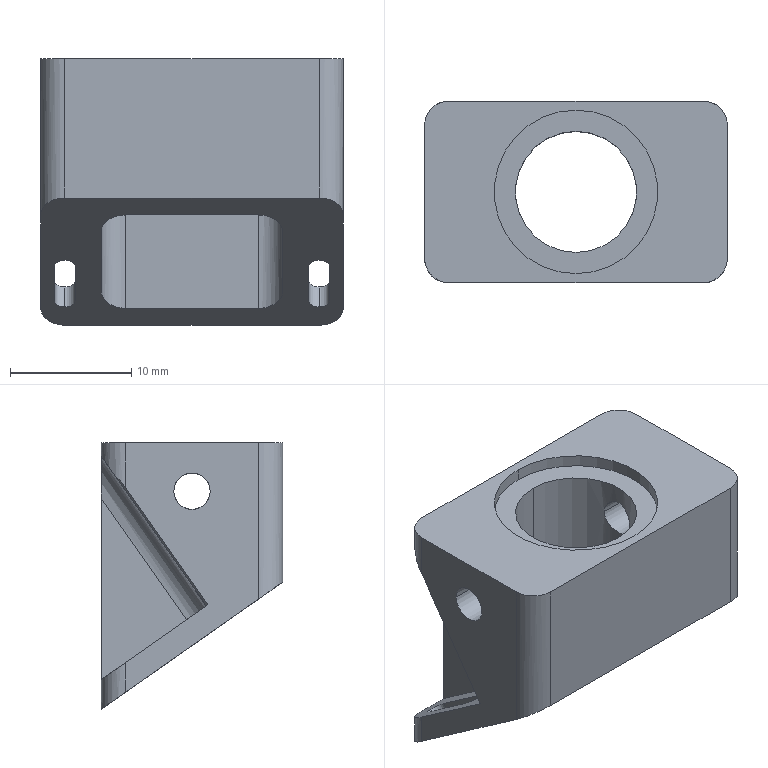NC program | NX | posted with a generic post | part box 25 x 15 x 22 mm
Whole program, first 1577 of 1758 lines:
N10 G17 G21 G94 G90
(FACE_MILLING , TOOL : D40面刀)
N12 T01 M6
N14 G54
N16 G17 G0 G90 X34.5 Y0. S3500 M3
N18 G43 Z20. H1
N20 Z3.
N22 G94 G1 Z0. F480.
N24 X32.5
N26 X-32.5 F800.
N28 X-34.5
N30 Z3.
N32 G0 Z20.
N34 M5
(SPOT_DRILLING , TOOL : D4点钻)
N36 T04 M6
N38 G54
N40 G17 G0 G90 X0. Y0. S2000 M3
N42 G43 Z20. H4
N44 G94 G82 G99 Z-2. F250. P200 R2.
N46 G80
N48 G0 X0. Y0. Z20.
N50 M5
(SPOT_DRILLING_COPY , TOOL : 9.5钻头)
N52 T05 M6
N54 G54
N56 G17 G0 G90 X0. Y0. S1600 M3
N58 G43 Z20. H5
N60 G94 G83 G98 Z-25. F250. Q3. R2.
N62 G80
N64 G0 X0. Y0. Z20.
N66 M5
(PLANAR_MILL , TOOL : D8开粗)
N68 T02 M6
N70 G54
N72 G17 G0 G90 X-21.239 Y-8.5 S4500 M3
N74 G43 Z20. H2
N76 Z-20.3
N78 G94 G1 Z-22.3 F900.
N80 X-20.65
N82 G3 X-17.65 Y-5.5 R3.
N84 G1 Y5.5 F1500.
N86 G2 X-10.5 Y12.65 R7.15
N88 G1 X10.5
N90 G2 X17.65 Y5.5 R7.15
N92 G1 Y-5.5
N94 G2 X10.5 Y-12.65 R7.15
N96 G1 X-10.5
N98 G2 X-17.65 Y-5.5 R7.15
N100 G3 X-20.65 Y-2.5 R3.
N102 G1 X-19.65 Y-8.5
N104 G3 X-16.65 Y-5.5 R3. F900.
N106 G1 Y5.5 F1500.
N108 G2 X-10.5 Y11.65 R6.15
N110 G1 X10.5
N112 G2 X16.65 Y5.5 R6.15
N114 G1 Y-5.5
N116 G2 X10.5 Y-11.65 R6.15
N118 G1 X-10.5
N120 G2 X-16.65 Y-5.5 R6.15
N122 G3 X-19.65 Y-2.5 R3.
N124 G1 X-21.65
N126 Z-20.3
N128 G0 Z20.
(PLANAR_MILL_COPY_2 , TOOL : D8开粗)
N130 X0. Y0.
N132 Z-0.9
N134 G1 X-1.247 Y0.069 F600.
N136 G3 X-2.116 Y-1.511 R1.
N138 X1.511 Y-2.116 R2.6 F1000.
N140 X-2.116 Y-1.511 R-2.6
N142 X-0.34 Y-1.202 R1.
N144 G1 X0. Y0.
N146 G0 Z20.
N148 M5
(PLANAR_MILL_COPY_1 , TOOL : D8精光)
N150 T03 M6
N152 G54
N154 G17 G0 G90 X-20.236 Y-8.465 S4500 M3
N156 G43 Z20. H3
N158 Z-20.3
N160 G94 G1 Z-22.3 F480.
N162 G41 X-20.039 Y-8.5 D3
N164 X-19.5
N166 G3 X-16.5 Y-5.5 R3.
N168 G1 Y5.5 F800.
N170 G2 X-10.5 Y11.5 R6.
N172 G1 X10.5
N174 G2 X16.5 Y5.5 R6.
N176 G1 Y-5.5
N178 G2 X10.5 Y-11.5 R6.
N180 G1 X-10.5
N182 G2 X-16.5 Y-5.5 R6.
N184 G3 X-19.5 Y-2.5 R3.
N186 G1 X-20.5
N188 G40
N190 X-20.697 Y-2.535
N192 Z-20.3
N194 G0 Z20.
(PLANAR_MILL_COPY_1_COPY , TOOL : D8精光)
N196 X-1.569 Y0.065 S3500
N198 Z1.
N200 G1 Z-1. F480.
N202 G41 X-1.75 Y-0.021
N204 X-2.005 Y-0.203
N206 G3 X-2.238 Y-1.598 R1.
N208 X1.598 Y-2.238 R2.75 F800.
N210 X-2.238 Y-1.598 R-2.75
N212 X-0.843 Y-1.831 R1.
N214 G1 X-0.587 Y-1.648
N216 G40
N218 X-0.447 Y-1.506
N220 Z1.
N222 G0 Z20.
N224 M5
(PLANAR_MILL_COPY , TOOL : R1)
N226 T13 M6
N228 G54
N230 G17 G0 G90 X-14.363 Y-6.465 S4500 M3
N232 G43 Z20. H13
N234 Z0.5
N236 G94 G1 Z-0.5 F600.
N238 G41 X-14.166 Y-6.5 D13
N240 G3 X-13.166 Y-5.5 R1.
N242 G1 Y5.5 F1000.
N244 G2 X-10.5 Y8.166 R2.666
N246 G1 X10.5
N248 G2 X13.166 Y5.5 R2.666
N250 G1 Y-5.5
N252 G2 X10.5 Y-8.166 R2.666
N254 G1 X-10.5
N256 G2 X-13.166 Y-5.5 R2.666
N258 G3 X-14.166 Y-4.5 R1.
N260 G40
N262 G1 X-14.363 Y-4.535
N264 Z0.5
N266 G0 Z20.
(PLANAR_MILL_COPY_COPY , TOOL : R1)
N268 X-4.456 Y-1.997
N270 Z0.5
N272 G1 Z-0.5 F600.
N274 G41 X-4.637 Y-2.083
N276 G3 X-4.869 Y-3.478 R1.
N278 X3.478 Y-4.869 R5.984 F1000.
N280 X-4.869 Y-3.478 R-5.984
N282 X-3.474 Y-3.711 R1.
N284 G40
N286 G1 X-3.334 Y-3.568
N288 Z0.5
N290 G0 Z20.
(PLANAR_MILL_COPY_COPY_COPY , TOOL : R1)
N292 X-2.989 Y-0.949
N294 Z-0.5
N296 G1 Z-1.5 F600.
N298 G41 X-3.169 Y-1.035
N300 X-3.294 Y-1.124
N302 G3 X-3.527 Y-2.519 R1.
N304 X2.519 Y-3.527 R4.334 F1000.
N306 X-3.527 Y-2.519 R-4.334
N308 X-2.132 Y-2.752 R1.
N310 G1 X-2.007 Y-2.662
N312 G40
N314 X-1.867 Y-2.52
N316 Z-0.5
N318 G0 Z20.
N320 M5
(ADAPTIVE_MILLING , TOOL : D4开粗)
N322 T08 M6
N324 G54
N326 G17 G0 G90 X-15.582 Y11.515 S5500 M3
N328 G43 Z13.982 H8
N330 Z-12.918
N332 G94 G1 Z-15.918 F1200.
N334 X-15.232 Y11.543 F2000.
N336 X-14.884 Y11.588
N338 G3 X-14.6 Y11.973 R0.405
N340 G2 X-14.386 Y13.882 R6.031
N342 G3 X-14.206 Y17.495 R26.504
N344 G2 X-14.176 Y23.935 R463.382
N346 X-12.751 Y25.861 R2.494
N348 X-9.948 Y26.517 R7.049
N350 G3 X-8.631 Y26.644 R8.532
N352 X-8.035 Y27.2 R0.873
N354 X-8.3 Y27.648 R0.402
N356 G1 X-9.027 Y27.947 Z-15.818
N358 X-9.377 Y28.086
N360 X-9.472 Y28.094
N362 X-9.566 Y28.084
N364 X-12.581 Y27.326
N366 G3 X-13.515 Y26.843 R3.15
N368 X-14.641 Y25.821 R6.151
N370 X-15.3 Y24.545 R4.061
N372 X-15.515 Y23.303 R4.524
N374 G1 X-15.776 Y14.49
N376 X-15.745 Y14.376
N378 X-15.44 Y13.687
N380 X-15.337 Y13.448 Z-15.851
N382 X-15.219 Y13.215 Z-15.884
N384 G3 X-15.006 Y13.067 Z-15.918 R0.413
N386 X-14.528 Y13.299 R0.401
N388 X-13.886 Y16.065 R6.646
N390 X-13.786 Y22.835 R158.507
N392 G2 X-11.974 Y25.361 R3.146
N394 X-9.563 Y26.059 R8.306
N396 G3 X-8.14 Y26.72 R2.469
N398 X-8.021 Y26.99 R0.72
N400 X-8.231 Y27.36 R0.402
N402 X-8.555 Y27.414 Z-15.876 R0.726
N404 G1 X-9.008 Y27.433 Z-15.818
N406 X-9.672 Y27.457
N408 G3 X-11.285 Y27.007 R13.359
N410 G1 X-12.09 Y26.663
N412 X-12.882 Y26.289
N414 G3 X-14.037 Y25.322 R3.789
N416 X-14.633 Y24.272 R3.101
N418 X-14.988 Y22.607 R5.297
N420 G1 X-15.203 Y15.337
N422 X-15.089 Y14.429
N424 X-15.058 Y14.17 Z-15.851
N426 X-15.011 Y13.913 Z-15.884
N428 G3 X-14.849 Y13.711 Z-15.918 R0.413
N430 X-14.319 Y13.806 R0.4
N432 X-13.657 Y15.437 R3.226
N434 X-13.409 Y19.6 R28.394
N436 G2 X-13.352 Y22.236 R29.078
N438 X-11.199 Y24.963 R3.652
N440 X-9.138 Y25.755 R37.205
N442 G3 X-8.062 Y26.523 R2.381
N444 G1 X-8.011 Y26.711
N446 X-8.035 Y27.51
N448 G3 X-8.323 Y27.882 R0.401
N450 X-8.731 Y27.778 Z-15.862 R0.439
N452 G1 X-9.011 Y27.575 Z-15.818
N454 X-9.743 Y27.053
N456 X-11.542 Y26.149
N458 G3 X-12.882 Y25.289 R8.835
N460 X-14.07 Y23.854 R5.135
N462 X-14.46 Y22.55 R3.909
N464 G1 X-14.597 Y21.332
N466 X-14.702 Y20.111
N468 X-15.021 Y15.535
N470 X-14.908 Y14.669
N472 X-14.835 Y14.167 Z-15.882
N474 G3 X-14.668 Y13.95 Z-15.918 R0.421
N476 X-14.136 Y14.044 R0.4
N478 X-13.297 Y15.907 R3.444
N480 X-13.017 Y19.958 R26.017
N482 G2 X-12.835 Y22.037 R7.857
N484 X-10.779 Y24.467 R4.194
N486 G3 X-8.738 Y25.553 R56.293
N488 X-8.016 Y26.28 R1.703
N490 G1 X-8.011 Y26.726
N492 G3 X-8.235 Y27.073 R0.402
N494 X-8.59 Y27.08 Z-15.871 R0.456
N496 G1 X-8.996 Y26.969 Z-15.818
N498 X-9.693 Y26.776
N500 X-9.779 Y26.726
N502 X-12.528 Y24.664
N504 G3 X-13.045 Y24.146 R2.528
N506 G1 X-13.309 Y23.777
N508 X-13.553 Y23.394
N510 G3 X-14.007 Y22.147 R4.286
N512 G1 X-14.119 Y21.57
N514 X-14.203 Y20.989
N516 X-14.8 Y15.787
N518 X-14.664 Y14.962
N520 X-14.573 Y14.461 Z-15.883
N522 G3 X-14.401 Y14.252 Z-15.918 R0.421
N524 X-13.913 Y14.312 R0.401
N526 X-13.062 Y15.769 R2.627
N528 X-12.648 Y19.389 R16.304
N530 G2 X-12.358 Y21.655 R7.242
N532 X-10.332 Y24.068 R4.979
N534 G3 X-9.827 Y24.449 R2.094
N536 G1 X-9.702 Y24.694
N538 X-9.242 Y25.155
N540 G3 X-8.192 Y25.755 R4.982
N542 X-8.002 Y26.419 R0.706
N544 X-8.827 Y26.619 R0.44
N546 G1 X-9.144 Y26.034
N548 G3 X-8.661 Y25.45 R0.44
N550 X-7.998 Y25.905 R0.683
N552 G1 X-7.995 Y26.169
N554 G3 X-8.812 Y26.381 R0.44
N556 G1 X-8.991 Y26.07
N558 G3 X-8.513 Y25.474 R0.44
N560 X-7.989 Y25.983 R0.482
N562 X-8.208 Y26.328 R0.402
N564 G1 X-8.364 Y26.373 Z-15.897
N566 X-8.524 Y26.394 Z-15.877
N568 X-8.981 Y26.458 Z-15.818
N570 X-9.464 Y26.52
N572 G3 X-9.697 Y26.44 R0.421
N574 G1 X-11.459 Y25.112
N576 G3 X-12.701 Y23.628 R5.464
N578 X-13.537 Y21.863 R8.092
N580 X-13.73 Y20.909 R5.162
N582 G1 X-14.214 Y16.147
N584 X-14.336 Y15.254
N586 X-14.374 Y14.996 Z-15.851
N588 X-14.396 Y14.736 Z-15.884
N590 G3 X-14.292 Y14.499 Z-15.918 R0.413
N592 X-13.755 Y14.452 R0.4
N594 X-12.779 Y15.863 R2.479
N596 X-12.305 Y18.84 R12.275
N598 G2 X-11.91 Y21.242 R7.668
N600 X-10.315 Y23.409 R5.937
N602 G3 X-9.998 Y24.113 R0.903
N604 G1 X-9.816 Y24.47
N606 G3 X-10.622 Y24.821 R-0.44
N608 G1 X-10.798 Y24.339
N610 X-11.068 Y23.601 Z-15.818
N612 X-14.044 Y15.477
N614 X-14.12 Y15.277 Z-15.845
N616 X-14.18 Y15.071 Z-15.872
N618 G3 X-14.087 Y14.738 Z-15.918 R0.444
N620 X-13.477 Y14.665 R0.44
N622 X-12.524 Y15.881 R2.225
N624 X-11.983 Y18.413 R9.705
N626 G2 X-11.402 Y21.032 R7.915
N628 X-10.256 Y22.791 R10.278
N630 G3 X-10.1 Y23.471 R0.899
N632 G1 X-10.053 Y23.767
N634 G3 X-10.755 Y24.185 R0.44
N636 X-10.94 Y23.874 Z-15.871 R0.583
N638 G1 X-11.078 Y23.481 Z-15.818
N640 X-13.825 Y15.618
N642 X-13.899 Y15.413 Z-15.846
N644 X-13.958 Y15.203 Z-15.873
N646 G3 X-13.866 Y14.876 Z-15.918 R0.445
N648 X-13.354 Y14.744 R0.441
N650 X-12.319 Y15.792 R1.908
N652 X-11.665 Y18.152 R8.173
N654 G2 X-10.274 Y21.968 R8.667
N656 G3 X-10.1 Y22.369 R1.883
N658 G1 Y23.169
N660 G3 X-10.666 Y23.591 R0.44
N662 X-10.98 Y23.245 Z-15.856 R0.474
N664 G1 X-11.078 Y22.964 Z-15.818
N666 X-13.638 Y15.698
N668 X-13.713 Y15.492 Z-15.846
N670 X-13.773 Y15.281 Z-15.874
N672 G3 X-13.684 Y14.956 Z-15.918 R0.445
N674 X-13.169 Y14.82 R0.441
N676 X-12.022 Y15.894 R2.011
N678 X-11.425 Y17.627 R7.32
N680 G2 X-10.131 Y21.34 R13.088
N682 G3 X-10.1 Y22.37 R4.674
N684 X-10.674 Y22.789 R0.44
N686 X-10.98 Y22.442 Z-15.856 R0.475
N688 G1 X-11.078 Y22.157 Z-15.818
N690 X-13.248 Y15.859
N692 X-13.328 Y15.638 Z-15.848
N694 X-13.388 Y15.411 Z-15.878
N696 G3 X-13.307 Y15.113 Z-15.918 R0.447
N698 X-12.894 Y14.934 R0.442
N700 X-11.949 Y15.626 R1.519
N702 X-11.067 Y17.679 R6.627
N704 G2 X-10.105 Y20.411 R25.158
N706 G1 X-10.1 Y21.496
N708 G3 X-10.638 Y21.925 R0.44
N710 X-10.976 Y21.588 Z-15.854 R0.47
N712 G1 X-11.078 Y21.323 Z-15.818
N714 X-13.178 Y15.882
N716 X-13.267 Y15.662 Z-15.848
N718 X-13.336 Y15.435 Z-15.878
N720 G3 X-13.271 Y15.138 Z-15.918 R0.448
N722 X-12.844 Y14.941 R0.442
N724 X-11.671 Y15.673 R1.616
N726 X-10.738 Y17.593 R7.135
N728 G1 X-10.1 Y19.345
N730 Y20.495
N732 G3 X-10.609 Y20.93 R0.44
N734 X-10.974 Y20.598 Z-15.852 R0.471
N736 G1 X-11.078 Y20.354 Z-15.818
N738 X-12.959 Y15.926
N740 X-13.056 Y15.705 Z-15.848
N742 X-13.135 Y15.478 Z-15.879
N744 G3 X-13.085 Y15.185 Z-15.918 R0.449
N746 X-12.646 Y14.967 R0.441
N748 X-11.405 Y15.688 R1.707
N750 X-10.252 Y17.877 R8.845
N752 G1 X-10.1 Y18.301
N754 Y19.351
N756 G3 X-10.57 Y19.79 R0.44
N758 X-10.967 Y19.479 Z-15.85 R0.467
N760 G1 X-11.078 Y19.252 Z-15.818
N762 X-12.688 Y15.96
N764 X-12.795 Y15.75 Z-15.848
N766 X-12.883 Y15.531 Z-15.878
N768 G3 X-12.843 Y15.228 Z-15.918 R0.448
N770 X-12.398 Y15. R0.441
N772 X-11.204 Y15.615 R1.625
N774 X-10.107 Y17.404 R6.423
N776 G1 X-10.1 Y18.303
N778 G3 X-10.516 Y18.742 R0.44
N780 X-10.957 Y18.463 Z-15.847 R0.469
N782 G1 X-11.076 Y18.265 Z-15.818
N784 X-12.434 Y15.993
N786 X-12.559 Y15.79 Z-15.848
N788 X-12.667 Y15.578 Z-15.879
N790 G3 X-12.655 Y15.276 Z-15.918 R0.448
N792 X-12.249 Y15.006 R0.441
N794 X-10.978 Y15.562 R1.634
N796 X-10.113 Y16.743 R4.303
N798 G1 X-10.1 Y17.463
N800 G3 X-10.475 Y17.899 R0.441
N802 X-10.941 Y17.659 Z-15.847 R0.468
N804 G1 X-11.075 Y17.474 Z-15.818
N806 X-12.143 Y15.998
N808 X-12.392 Y15.644 Z-15.873
N810 G3 X-12.414 Y15.301 Z-15.918 R0.455
N812 X-11.999 Y15.006 R0.441
N814 X-10.681 Y15.561 R1.759
N816 X-10.11 Y16.291 R1.983
N818 G1 X-10.1 Y16.85
N820 G3 X-10.443 Y17.279 R0.441
N822 X-10.924 Y17.078 Z-15.847 R0.469
N824 G1 X-11.075 Y16.902 Z-15.818
N826 X-11.856 Y15.996
N828 X-12.125 Y15.674 Z-15.871
N830 G3 X-12.171 Y15.322 Z-15.918 R0.454
N832 X-11.749 Y15.006 R0.441
N834 X-10.123 Y15.903 R1.813
N836 X-10.1 Y16.358 R3.558
N838 X-10.411 Y16.779 R0.441
N840 X-10.895 Y16.628 Z-15.85 R0.466
N842 G1 X-11.076 Y16.456 Z-15.818
N844 X-11.561 Y15.995
N846 X-11.718 Y15.848 Z-15.845
N848 X-11.864 Y15.69 Z-15.873
N850 G3 X-11.929 Y15.351 Z-15.918 R0.444
N852 X-11.499 Y15.006 R0.441
N854 X-10.127 Y15.64 R1.381
N856 X-10.1 Y16.056 R2.236
N858 X-10.407 Y16.476 R0.441
N860 X-10.892 Y16.33 Z-15.85 R0.467
N862 G1 X-11.076 Y16.16 Z-15.818
N864 X-11.254 Y15.994
N866 X-11.413 Y15.85 Z-15.845
N868 X-11.56 Y15.695 Z-15.872
N870 G3 X-11.63 Y15.355 Z-15.918 R0.444
N872 X-11.199 Y15.006 R0.441
N874 X-10.149 Y15.411 R1.112
N876 X-10.1 Y15.778 R0.942
N878 X-10.839 Y16.101 R0.44
N880 G1 X-11.245 Y15.717
N882 G3 X-10.899 Y15.006 R0.44
N884 X-10.173 Y15.249 R0.793
N886 X-10.1 Y15.607 R0.686
N888 X-10.904 Y15.854 R0.44
N890 G1 X-10.998 Y15.718
N892 X-11.071 Y15.57
N894 G3 X-10.649 Y15.006 R0.44
N896 X-10.1 Y15.481 R0.455
N898 X-10.384 Y15.867 R0.405
N900 G1 X-11.082 Y16.084
N902 Z-12.918
N904 G0 Z13.982
N906 X7.338 Y28.069
N908 Z-12.918
N910 G1 Z-15.918 F1200.
N912 X6.703 Y27.909 F2000.
N914 G3 X6.399 Y27.485 R0.405
N916 X6.856 Y26.906 R0.533
N918 X9.472 Y26.634 R10.905
N920 G2 X11.69 Y26.569 R27.629
N922 X13.507 Y25.066 R2.578
N924 X14.119 Y22.199 R7.582
N926 X14.205 Y14.761 R179.701
N928 G1 X14.301 Y13.849
N930 G2 X14.6 Y12.755 R2.563
N932 G1 Y11.955
N934 G3 X15.274 Y11.664 R0.4
N936 X15.427 Y11.96 Z-15.875 R0.704
N938 G1 X15.579 Y12.382 Z-15.818
N940 X15.717 Y12.757
N942 X15.844 Y13.136
N944 X15.85 Y13.205
N946 X15.853 Y15.046
N948 X15.831 Y16.887
N950 G3 X15.546 Y20.554 R39.884
N952 G1 X15.114 Y23.963
N954 G3 X13.707 Y26.848 R5.665
N956 X12.675 Y27.51 R3.134
N958 X11.352 Y27.85 R5.189
N960 G1 X7.939 Y28.269
N962 X7.836 Y28.266
N964 X7.735 Y28.241
N966 X7.354 Y28.081
N968 X6.629 Y27.776 Z-15.918
N970 G3 X6.408 Y27.385 R0.401
N972 X6.807 Y26.807 R0.604
N974 X8.97 Y26.319 R5.727
N976 G2 X10.79 Y26.182 R20.503
N978 X13.072 Y24.165 R3.335
N980 X13.708 Y21.046 R9.166
N982 X13.812 Y15.325 R146.03
N984 G3 X13.932 Y14.314 R3.116
N986 G1 X14.338 Y13.76
N988 G3 X14.944 Y13.591 R0.4
N990 X15.112 Y13.953 Z-15.865 R0.442
N992 G1 X15.143 Y14.323 Z-15.818
N994 X15.222 Y15.291
N996 X15.202 Y16.722
N998 X15.162 Y18.153
N1000 X15.092 Y19.295
N1002 X14.99 Y20.435
N1004 X14.733 Y22.833
N1006 G3 X13.939 Y25.217 R7.439
N1008 X12.76 Y26.523 R4.348
N1010 X11.491 Y27.244 R5.443
N1012 X10.701 Y27.42 R4.004
N1014 G1 X10.053 Y27.501
N1016 X8.079 Y27.695
N1018 X7.386 Y27.68
N1020 X6.741 Y27.66 Z-15.9
N1022 X6.611 Y27.61 Z-15.918
N1024 G3 X6.42 Y27.235 R0.402
N1026 X6.908 Y26.601 R0.867
N1028 X9.124 Y25.98 R5.46
N1030 G2 X12.668 Y23.407 R3.907
N1032 X13.312 Y19.983 R10.693
N1034 X13.435 Y15.362 R599.298
N1036 G3 X13.629 Y14.558 R1.508
N1038 G1 X13.977 Y14.249
N1040 G3 X14.445 Y14.176 R0.401
N1042 X14.667 Y14.542 Z-15.861 R0.437
N1044 G1 X14.721 Y14.876 Z-15.818
N1046 X14.861 Y15.78
N1048 X14.862 Y16.802
N1050 X14.84 Y17.825
N1052 G3 X14.674 Y19.449 R16.845
N1054 G1 X14.24 Y22.236
N1056 G3 X13.649 Y24.203 R9.935
N1058 G1 X13.306 Y25.009
N1060 G3 X12.39 Y26.04 R2.832
N1062 X10.131 Y27.084 R8.287
N1064 G1 X8.072 Y27.655
N1066 X7.389 Y27.637
N1068 X6.741 Y27.61 Z-15.9
N1070 X6.614 Y27.559 Z-15.918
N1072 G3 X6.424 Y27.186 R0.402
N1074 X6.958 Y26.39 R1.047
N1076 X8.898 Y25.686 R5.264
N1078 G2 X12.312 Y22.635 R4.511
N1080 X12.924 Y18.898 R12.878
N1082 G3 X13.064 Y15.537 R68.24
N1084 X13.289 Y14.809 R1.429
N1086 G1 X13.365 Y14.744
N1088 G3 X13.766 Y14.745 R0.402
N1090 X13.971 Y15.072 Z-15.867 R0.449
N1092 G1 X14.061 Y15.448 Z-15.818
N1094 X14.246 Y16.228
N1096 G3 X14.208 Y18.728 R34.896
N1098 G1 X14.153 Y19.338
N1100 X14.084 Y19.947
N1102 X13.876 Y21.44
N1104 G3 X13.035 Y23.947 R8.586
N1106 X11.818 Y25.582 R7.801
N1108 X10.822 Y26.28 R3.806
N1110 X9.456 Y26.796 R5.492
N1112 G1 X8.164 Y27.096
N1114 X7.407 Y27.348
N1116 X6.896 Y27.513 Z-15.886
N1118 G3 X6.654 Y27.477 Z-15.918 R0.428
N1120 X6.432 Y27.086 R0.401
N1122 X7.037 Y26.131 R1.253
N1124 X8.709 Y25.436 R4.217
N1126 G2 X12.033 Y21.678 R5.414
N1128 X12.541 Y17.82 R16.66
N1130 G3 X12.744 Y15.485 R13.773
N1132 X13.108 Y14.846 R0.936
N1134 G2 X13.678 Y14.511 R1.44
N1136 G3 X14.202 Y14.544 R0.401
N1138 X14.307 Y14.958 Z-15.861 R0.437
N1140 G1 X14.261 Y15.294 Z-15.818
N1142 X13.992 Y17.34
N1144 X13.739 Y19.387
N1146 G3 X13.036 Y22.561 R16.894
N1148 X11.903 Y24.627 R6.798
N1150 X9.573 Y26.347 R6.279
N1152 G1 X8.179 Y26.949
N1154 X7.419 Y27.2
N1156 X6.908 Y27.363 Z-15.886
N1158 X6.784 Z-15.902
N1160 X6.666 Y27.327 Z-15.918
N1162 G3 X6.444 Y26.936 R0.401
N1164 X7.081 Y25.875 R1.383
N1166 X8.019 Y25.552 R1.122
N1168 G1 X8.414 Y25.49
N1170 G3 X8.918 Y25.987 R0.44
N1172 X8.624 Y26.347 Z-15.856 R0.475
N1174 G1 X8.36 Y26.489 Z-15.818
N1176 X7.435 Y26.985
N1178 X7.227 Y27.1 Z-15.848
N1180 X7.01 Y27.197 Z-15.878
N1182 G3 X6.709 Y27.169 Z-15.918 R0.448
N1184 X6.46 Y26.737 R0.441
N1186 X7.257 Y25.563 R1.357
N1188 G1 X7.668 Y25.552
N1190 G3 X8.102 Y25.915 R0.441
N1192 X7.876 Y26.387 Z-15.847 R0.468
N1194 G1 X7.695 Y26.528 Z-15.818
N1196 X7.456 Y26.712
N1198 X7.284 Y26.847 Z-15.846
N1200 X7.103 Y26.97 Z-15.874
N1202 G3 X6.765 Y26.987 Z-15.918 R0.445
N1204 X6.476 Y26.538 R0.441
N1206 X6.972 Y25.586 R1.069
N1208 X7.359 Y25.552 R1.533
N1210 X7.652 Y26.32 R0.44
N1212 G1 X7.168 Y26.744
N1214 G3 X6.492 Y26.338 R0.44
N1216 X6.775 Y25.619 R0.833
N1218 X7.124 Y25.552 R0.719
N1220 X7.392 Y26.341 R0.44
N1222 G1 X7.25 Y26.453
N1224 X7.092 Y26.542
N1226 G3 X6.513 Y26.089 R0.44
N1228 X6.998 Y25.552 R0.469
N1230 G2 X8.661 Y25.45 R6.715
N1232 G1 X9.242 Y25.155
N1234 G2 X11.918 Y19.814 R8.603
N1236 X12.237 Y16.398 R108.189
N1238 G3 X12.649 Y15.075 R3.
N1240 G1 X12.857 Y14.941
N1242 G3 X13.29 Y15.086 R0.442
N1244 X13.353 Y15.571 Z-15.852 R0.474
N1246 G1 X13.275 Y15.831 Z-15.818
N1248 X11.085 Y23.124
N1250 X10.859 Y23.876 Z-15.918
N1252 X10.68 Y24.484
N1254 X10.489 Y25.088
N1256 G3 X9.702 Y24.694 R-0.44
N1258 G2 X11.16 Y21.175 R19.871
N1260 X11.753 Y17.226 R23.84
N1262 G3 X12.19 Y15.386 R5.509
N1264 X12.894 Y14.934 R0.707
N1266 G1 X13.124 Y14.839
N1268 G3 X13.621 Y14.953 R0.441
N1270 X13.69 Y15.449 Z-15.85 R0.468
N1272 G1 X13.612 Y15.693 Z-15.818
N1274 X11.069 Y23.636
N1276 X10.824 Y24.383 Z-15.918
N1278 G3 X9.998 Y24.113 R0.44
N1280 X10.593 Y21.679 R16.069
N1282 G2 X11.345 Y17.319 R29.758
N1284 G3 X11.889 Y15.408 R5.352
N1286 X12.648 Y14.967 R0.793
N1288 X13.063 Y15.145 R0.442
N1290 X13.112 Y15.586 Z-15.859 R0.475
N1292 G1 X13.029 Y15.899 Z-15.818
N1294 X11.085 Y23.203
N1296 X10.929 Y23.766 Z-15.892
N1298 X10.877 Y23.852 Z-15.905
N1300 X10.81 Y23.926 Z-15.918
N1302 G3 X10.092 Y23.521 R0.44
N1304 X10.341 Y21.222 R9.938
N1306 G2 X11.001 Y17.084 R229.932
N1308 G3 X11.702 Y15.259 R4.203
N1310 X12.351 Y15.006 R0.637
N1312 X12.709 Y15.191 R0.443
N1314 X12.761 Y15.622 Z-15.86 R0.479
N1316 G1 X12.682 Y15.947 Z-15.818
N1318 X11.084 Y22.496
N1320 X11.018 Y22.778 Z-15.855
N1322 X10.937 Y23.056 Z-15.892
N1324 X10.882 Y23.142 Z-15.905
N1326 X10.811 Y23.216 Z-15.918
N1328 G3 X10.1 Y22.869 R0.44
N1330 X10.756 Y16.591 R24.263
N1332 X11.576 Y15.096 R2.956
N1334 X12.109 Y15.006 R0.769
N1336 X12.486 Y15.219 R0.442
N1338 X12.513 Y15.637 Z-15.863 R0.488
N1340 G1 X12.421 Y15.977 Z-15.818
N1342 X11.084 Y20.894
N1344 X10.943 Y21.396 Z-15.884
N1346 G3 X10.772 Y21.593 Z-15.918 R0.47
N1348 X10.1 Y21.219 R0.44
N1350 X10.14 Y18.057 R41.425
N1352 X10.925 Y15.477 R5.782
N1354 X11.506 Y15.006 R0.933
N1356 G1 X11.856
N1358 G3 X12.243 Y15.237 R0.442
N1360 X12.236 Y15.679 Z-15.859 R0.476
N1362 G1 X12.113 Y15.98 Z-15.818
N1364 X11.086 Y18.497
N1366 X11. Y18.715 Z-15.848
N1368 X10.895 Y18.926 Z-15.878
N1370 G3 X10.639 Y19.097 Z-15.918 R0.447
N1372 X10.1 Y18.669 R0.44
N1374 X10.148 Y16.743 R13.81
N1376 X10.981 Y15.091 R2.753
N1378 X11.513 Y15.006 R0.8
N1380 X11.91 Y15.257 R0.442
N1382 X11.86 Y15.726 Z-15.855 R0.472
N1384 G1 X11.717 Y15.979 Z-15.818
N1386 X11.087 Y17.094
N1388 X10.983 Y17.282 Z-15.845
N1390 X10.866 Y17.463 Z-15.873
N1392 G3 X10.553 Y17.609 Z-15.918 R0.444
N1394 X10.1 Y17.169 R0.44
N1396 X10.223 Y15.841 R3.676
N1398 X10.798 Y15.045 R1.501
N1400 X11.244 Y15.006 R1.288
N1402 X11.653 Y15.283 R0.441
N1404 X11.556 Y15.766 Z-15.852 R0.471
N1406 G1 X11.4 Y15.982 Z-15.818
N1408 X11.087 Y16.414
N1410 X10.964 Y16.586 Z-15.845
N1412 X10.829 Y16.749 Z-15.872
N1414 G3 X10.494 Y16.856 Z-15.918 R0.444
N1416 X10.1 Y16.419 R0.44
N1418 X10.398 Y15.205 R1.738
N1420 X10.99 Y15.006 R0.63
N1422 X11.406 Y15.303 R0.441
N1424 X11.276 Y15.788 Z-15.85 R0.468
N1426 G1 X11.109 Y15.982 Z-15.818
N1428 X11.088 Y16.007
N1430 X10.95 Y16.169 Z-15.845
N1432 X10.801 Y16.321 Z-15.872
N1434 G3 X10.462 Y16.402 Z-15.918 R0.444
N1436 X10.1 Y15.969 R0.441
N1438 X10.379 Y15.086 R1.022
N1440 X10.75 Y15.006 R0.656
N1442 X11.07 Y15.748 R0.44
N1444 G1 X10.808 Y16.017
N1446 G3 X10.1 Y15.669 R0.44
N1448 X10.39 Y15.037 R0.57
N1450 G1 X10.625 Y15.006
N1452 G3 X10.587 Y15.976 R-0.486
N1454 X10.1 Y15.469 R0.508
N1456 X10.492 Y15.011 R0.426
N1458 X10.942 Y15.291 R0.405
N1460 G1 X11.156 Y15.988
N1462 Z-12.918
N1464 G0 Z13.982
N1466 M5
(PLANAR_MILL_1_COPY , TOOL : D4精刀)
N1468 T06 M6
N1470 G54
N1472 G17 G0 G90 X-16.206 Y11.941 S4500 M3
N1474 G43 Z13.982 H6
N1476 Z-9.018
N1478 G94 G1 Z-10.018 F360.
N1480 G41 X-16.043 Y12.056 D6
N1482 X-13.921 Y14.177
N1484 X-13.771 Y14.327 F600.
N1486 G2 X-12.35 Y14.916 R2.01
N1488 G1 X-10.01
N1490 Y23.506
N1492 Y26.506
N1494 G40
N1496 X-10.045 Y26.703
N1498 Z-9.018
N1500 G0 Z13.982
N1502 X-16.199 Y11.934
N1504 Z-9.018
N1506 G1 Z-10.018 F360.
N1508 G41 X-16.036 Y12.049
N1510 X-13.914 Y14.17
N1512 X-13.764 Y14.32 F600.
N1514 G2 X-12.35 Y14.906 R2.
N1516 G1 X-10.
N1518 Y23.506
N1520 Y26.506
N1522 G40
N1524 X-10.035 Y26.703
N1526 Z-9.018
N1528 G0 Z13.982
N1530 X10.045
N1532 Z-9.018
N1534 G1 Z-10.018 F360.
N1536 G41 X10.01 Y26.506
N1538 Y23.506
N1540 Y14.916 F600.
N1542 X12.35
N1544 G2 X13.771 Y14.327 R2.01
N1546 G1 X13.921 Y14.177
N1548 X16.043 Y12.056
N1550 G40
N1552 X16.206 Y11.941
N1554 Z-9.018
N1556 G0 Z13.982
N1558 X10.035 Y26.703
N1560 Z-9.018
N1562 G1 Z-10.018 F360.
N1564 G41 X10. Y26.506
N1566 Y23.506
N1568 Y14.906 F600.
N1570 X12.35
N1572 G2 X13.764 Y14.32 R2.
N1574 G1 X13.914 Y14.17
N1576 X16.036 Y12.049
N1578 G40
N1580 X16.199 Y11.934
N1582 Z-9.018
N1584 G0 Z13.982
(PLANAR_MILL_1_COPY_COPY , TOOL : D4精刀)
N1586 X-17.614 Y13.348
N1588 Z-15.018
N1590 G1 Z-16.018 F360.
N1592 G41 X-17.45 Y13.463
N1594 X-15.328 Y15.584
N1596 X-15.178 Y15.734 F600.
N1598 G2 X-12.35 Y16.906 R4.
N1600 G1 X-12.
N1602 Y23.506
N1604 Y26.506
N1606 G40
N1608 X-12.035 Y26.703
N1610 Z-15.018
N1612 G0 Z13.982
N1614 X-16.199 Y11.934
N1616 Z-15.018
N1618 G1 Z-16.018 F360.
N1620 G41 X-16.036 Y12.049
N1622 X-13.914 Y14.17
N1624 X-13.764 Y14.32 F600.
N1626 G2 X-12.35 Y14.906 R2.
N1628 G1 X-10.
N1630 Y23.506
N1632 Y26.506
N1634 G40
N1636 X-10.035 Y26.703
N1638 Z-15.018
N1640 G0 Z13.982
N1642 X12.035
N1644 Z-15.018
N1646 G1 Z-16.018 F360.
N1648 G41 X12. Y26.506
N1650 Y23.506
N1652 Y16.906 F600.
N1654 X12.35
N1656 G2 X15.178 Y15.734 R4.
N1658 G1 X15.328 Y15.584
N1660 X17.45 Y13.463
N1662 G40
N1664 X17.614 Y13.348
N1666 Z-15.018
N1668 G0 Z13.982
N1670 X10.035 Y26.703
N1672 Z-15.018
N1674 G1 Z-16.018 F360.
N1676 G41 X10. Y26.506
N1678 Y23.506
N1680 Y14.906 F600.
N1682 X12.35
N1684 G2 X13.764 Y14.32 R2.
N1686 G1 X13.914 Y14.17
N1688 X16.036 Y12.049
N1690 G40
N1692 X16.199 Y11.934
N1694 Z-15.018
N1696 G0 Z13.982
(PLANAR_MILL_1_COPY_COPY_COPY , TOOL : D4精刀)
N1698 X-17.614 Y13.348
N1700 Z-15.018
N1702 G1 Z-16.018 F360.
N1704 G41 X-17.45 Y13.463
N1706 X-15.328 Y15.584
N1708 X-15.178 Y15.734 F600.
N1710 G2 X-12.35 Y16.906 R4.
N1712 G1 X-12.
N1714 Y23.506
N1716 Y26.506
N1718 G40
N1720 X-12.035 Y26.703
N1722 Z-15.018
N1724 G0 Z13.982
N1726 X-16.199 Y11.934
N1728 Z-15.018
N1730 G1 Z-16.018 F360.
N1732 G41 X-16.036 Y12.049
N1734 X-13.914 Y14.17
N1736 X-13.764 Y14.32 F600.
N1738 G2 X-12.35 Y14.906 R2.
N1740 G1 X-10.
N1742 Y23.506
N1744 Y26.506
N1746 G40
N1748 X-10.035 Y26.703
N1750 Z-15.018
N1752 G0 Z13.982
N1754 X12.035
N1756 Z-15.018
N1758 G1 Z-16.018 F360.
N1760 G41 X12. Y26.506
N1762 Y23.506
N1764 Y16.906 F600.
N1766 X12.35
N1768 G2 X15.178 Y15.734 R4.
N1770 G1 X15.328 Y15.584
N1772 X17.45 Y13.463
N1774 G40
N1776 X17.614 Y13.348
N1778 Z-15.018
N1780 G0 Z13.982
N1782 X10.035 Y26.703
N1784 Z-15.018
N1786 G1 Z-16.018 F360.
N1788 G41 X10. Y26.506
N1790 Y23.506
N1792 Y14.906 F600.
N1794 X12.35
N1796 G2 X13.764 Y14.32 R2.
N1798 G1 X13.914 Y14.17
N1800 X16.036 Y12.049
N1802 G40
N1804 X16.199 Y11.934
N1806 Z-15.018
N1808 G0 Z13.982
N1810 M5
(PLANAR_MILL_1 , TOOL : D40面刀)
N1812 T01 M6
N1814 G54
N1816 G17 G0 G90 X35.5 Y0.688 S3500 M3
N1818 G43 Z20. H1
N1820 Z10.586
N1822 G94 G1 Z8.586 F1500.
N1824 X10.5
N1826 X-10.5
N1828 X-35.5
N1830 Z10.586
N1832 G0 Z13.
N1834 X35.5
N1836 Z9.171
N1838 G1 Z7.171
N1840 X10.5
N1842 X-10.5
N1844 X-35.5
N1846 Z9.171
N1848 G0 Z11.586
N1850 X35.5
N1852 Z7.757
N1854 G1 Z5.757
N1856 X10.5
N1858 X-10.5
N1860 X-35.5
N1862 Z7.757
N1864 G0 Z10.171
N1866 X35.5
N1868 Z6.343
N1870 G1 Z4.343
N1872 X10.5
N1874 X-10.5
N1876 X-35.5
N1878 Z6.343
N1880 G0 Z8.757
N1882 X35.5
N1884 Z4.929
N1886 G1 Z2.929
N1888 X10.5
N1890 X-10.5
N1892 X-35.5
N1894 Z4.929
N1896 G0 Z7.343
N1898 X35.5
N1900 Z3.514
N1902 G1 Z1.514
N1904 X10.5
N1906 X-10.5
N1908 X-35.5
N1910 Z3.514
N1912 G0 Z5.929
N1914 X35.5
N1916 Z2.1
N1918 G1 Z0.1
N1920 X10.5
N1922 X-10.5
N1924 X-35.5
N1926 Z2.1
N1928 G0 Z20.
(PLANAR_MILL_1_COPY_1 , TOOL : D40面刀)
N1930 X33.5
N1932 Z3.
N1934 G1 Z0. F800.
N1936 X10.5
N1938 X-10.5
N1940 X-33.5
N1942 Z3.
N1944 G0 Z20.
N1946 M5
(PLANAR_MILL_2 , TOOL : D1精刀)
N1948 T07 M6
N1950 G54
N1952 G17 G0 G90 X-10.555 Y-3.256 S4500 M3
N1954 G43 Z20. H7
N1956 Z0.2
N1958 G94 G1 X-10.638 Y-3.288 Z0.198 F480.
N1960 X-10.712 Y-3.362 Z0.195
N1962 X-10.75 Y-3.461 Z0.192
N1964 Y-8.539 Z0.059
N1966 X-10.712 Y-8.638 Z0.056
N1968 X-10.638 Y-8.712 Z0.054
N1970 X-10.539 Y-8.75 Z0.051
N1972 X-10.461 Z0.049
N1974 X-10.362 Y-8.712 Z0.046
N1976 X-10.288 Y-8.638 Z0.043
N1978 X-10.25 Y-8.539 Z0.041
N1980 Y-3.461 Z-0.092
N1982 X-10.288 Y-3.362 Z-0.095
N1984 X-10.362 Y-3.288 Z-0.098
N1986 X-10.461 Y-3.25 Z-0.101
N1988 X-10.539 Z-0.103
N1990 X-10.638 Y-3.288 Z-0.106
N1992 X-10.712 Y-3.362 Z-0.108
N1994 X-10.75 Y-3.461 Z-0.111
N1996 Y-8.539 Z-0.244
N1998 X-10.712 Y-8.638 Z-0.247
N2000 X-10.638 Y-8.712 Z-0.25
N2002 X-10.539 Y-8.75 Z-0.252
N2004 X-10.461 Z-0.254
N2006 X-10.362 Y-8.712 Z-0.257
N2008 X-10.288 Y-8.638 Z-0.26
N2010 X-10.25 Y-8.539 Z-0.263
N2012 Y-3.461 Z-0.396
N2014 X-10.288 Y-3.362 Z-0.398
N2016 X-10.362 Y-3.288 Z-0.401
N2018 X-10.461 Y-3.25 Z-0.404
N2020 X-10.539 Z-0.406
N2022 X-10.638 Y-3.288 Z-0.409
N2024 X-10.712 Y-3.362 Z-0.412
N2026 X-10.75 Y-3.461 Z-0.414
N2028 Y-8.539 Z-0.547
N2030 X-10.712 Y-8.638 Z-0.55
N2032 X-10.638 Y-8.712 Z-0.553
N2034 X-10.539 Y-8.75 Z-0.556
N2036 X-10.461 Z-0.558
N2038 X-10.362 Y-8.712 Z-0.56
N2040 X-10.288 Y-8.638 Z-0.563
N2042 X-10.25 Y-8.539 Z-0.566
N2044 Y-3.461 Z-0.699
N2046 X-10.288 Y-3.362 Z-0.702
N2048 X-10.362 Y-3.288 Z-0.704
N2050 X-10.461 Y-3.25 Z-0.707
N2052 X-10.539 Z-0.709
N2054 X-10.638 Y-3.288 Z-0.712
N2056 X-10.712 Y-3.362 Z-0.715
N2058 X-10.75 Y-3.461 Z-0.717
N2060 Y-8.539 Z-0.85
N2062 X-10.712 Y-8.638 Z-0.853
N2064 X-10.638 Y-8.712 Z-0.856
N2066 X-10.539 Y-8.75 Z-0.859
N2068 X-10.461 Z-0.861
N2070 X-10.362 Y-8.712 Z-0.864
N2072 X-10.288 Y-8.638 Z-0.866
N2074 X-10.25 Y-8.539 Z-0.869
N2076 Y-3.461 Z-1.002
N2078 X-10.288 Y-3.362 Z-1.005
N2080 X-10.362 Y-3.288 Z-1.008
N2082 X-10.461 Y-3.25 Z-1.01
N2084 X-10.539 Z-1.012
N2086 X-10.638 Y-3.288 Z-1.015
N2088 X-10.712 Y-3.362 Z-1.018
N2090 X-10.75 Y-3.461 Z-1.021
N2092 Y-8.539 Z-1.154
N2094 X-10.712 Y-8.638 Z-1.156
N2096 X-10.638 Y-8.712 Z-1.159
N2098 X-10.539 Y-8.75 Z-1.162
N2100 X-10.461 Z-1.164
N2102 X-10.362 Y-8.712 Z-1.167
N2104 X-10.288 Y-8.638 Z-1.17
N2106 X-10.25 Y-8.539 Z-1.172
N2108 Y-3.461 Z-1.305
N2110 X-10.288 Y-3.362 Z-1.308
N2112 X-10.362 Y-3.288 Z-1.311
N2114 X-10.461 Y-3.25 Z-1.314
N2116 X-10.539 Z-1.316
N2118 X-10.638 Y-3.288 Z-1.318
N2120 X-10.712 Y-3.362 Z-1.321
N2122 X-10.75 Y-3.461 Z-1.324
N2124 Y-8.539 Z-1.457
N2126 X-10.712 Y-8.638 Z-1.46
N2128 X-10.638 Y-8.712 Z-1.462
N2130 X-10.539 Y-8.75 Z-1.465
N2132 X-10.461 Z-1.467
N2134 X-10.362 Y-8.712 Z-1.47
N2136 X-10.288 Y-8.638 Z-1.473
N2138 X-10.25 Y-8.539 Z-1.476
N2140 Y-3.461 Z-1.608
N2142 X-10.288 Y-3.362 Z-1.611
N2144 X-10.362 Y-3.288 Z-1.614
N2146 X-10.461 Y-3.25 Z-1.617
N2148 X-10.539 Z-1.619
N2150 X-10.638 Y-3.288 Z-1.622
N2152 X-10.712 Y-3.362 Z-1.624
N2154 X-10.75 Y-3.461 Z-1.627
N2156 Y-8.539 Z-1.76
N2158 X-10.712 Y-8.638 Z-1.763
N2160 X-10.638 Y-8.712 Z-1.766
N2162 X-10.539 Y-8.75 Z-1.768
N2164 X-10.461 Z-1.77
N2166 X-10.362 Y-8.712 Z-1.773
N2168 X-10.288 Y-8.638 Z-1.776
N2170 X-10.25 Y-8.539 Z-1.779
N2172 Y-3.461 Z-1.912
N2174 X-10.288 Y-3.362 Z-1.914
N2176 X-10.362 Y-3.288 Z-1.917
N2178 X-10.461 Y-3.25 Z-1.92
N2180 X-10.539 Z-1.922
N2182 X-10.638 Y-3.288 Z-1.925
N2184 X-10.712 Y-3.362 Z-1.928
N2186 X-10.75 Y-3.461 Z-1.93
N2188 Y-8.539 Z-2.063
N2190 X-10.712 Y-8.638 Z-2.066
N2192 X-10.638 Y-8.712 Z-2.069
N2194 X-10.539 Y-8.75 Z-2.072
N2196 X-10.461 Z-2.074
N2198 X-10.362 Y-8.712 Z-2.076
N2200 X-10.288 Y-8.638 Z-2.079
N2202 X-10.25 Y-8.539 Z-2.082
N2204 Y-3.461 Z-2.215
N2206 X-10.288 Y-3.362 Z-2.218
N2208 X-10.362 Y-3.288 Z-2.22
N2210 X-10.461 Y-3.25 Z-2.223
N2212 X-10.539 Z-2.225
N2214 X-10.638 Y-3.288 Z-2.228
N2216 X-10.712 Y-3.362 Z-2.231
N2218 X-10.75 Y-3.461 Z-2.234
N2220 Y-6. Z-2.3
N2222 Y-8.5 F800.
N2224 G3 X-10.5 Y-8.75 R0.25
N2226 X-10.25 Y-8.5 R0.25
N2228 G1 Y-3.5
N2230 G3 X-10.5 Y-3.25 R0.25
N2232 X-10.75 Y-3.5 R0.25
N2234 G1 Y-6.
N2236 X-10.25
N2238 Z0.7
N2240 X10.555 Y-8.744 F8000.
N2242 G0 Z0.2
N2244 G1 X10.638 Y-8.712 Z0.198 F480.
N2246 X10.712 Y-8.638 Z0.195
N2248 X10.75 Y-8.539 Z0.192
N2250 Y-3.461 Z0.059
N2252 X10.712 Y-3.362 Z0.056
N2254 X10.638 Y-3.288 Z0.054
N2256 X10.539 Y-3.25 Z0.051
N2258 X10.461 Z0.049
N2260 X10.362 Y-3.288 Z0.046
N2262 X10.288 Y-3.362 Z0.043
N2264 X10.25 Y-3.461 Z0.041
N2266 Y-8.539 Z-0.092
N2268 X10.288 Y-8.638 Z-0.095
N2270 X10.362 Y-8.712 Z-0.098
N2272 X10.461 Y-8.75 Z-0.101
N2274 X10.539 Z-0.103
N2276 X10.638 Y-8.712 Z-0.106
N2278 X10.712 Y-8.638 Z-0.108
N2280 X10.75 Y-8.539 Z-0.111
N2282 Y-3.461 Z-0.244
N2284 X10.712 Y-3.362 Z-0.247
N2286 X10.638 Y-3.288 Z-0.25
N2288 X10.539 Y-3.25 Z-0.252
N2290 X10.461 Z-0.254
N2292 X10.362 Y-3.288 Z-0.257
N2294 X10.288 Y-3.362 Z-0.26
N2296 X10.25 Y-3.461 Z-0.263
N2298 Y-8.539 Z-0.396
N2300 X10.288 Y-8.638 Z-0.398
N2302 X10.362 Y-8.712 Z-0.401
N2304 X10.461 Y-8.75 Z-0.404
N2306 X10.539 Z-0.406
N2308 X10.638 Y-8.712 Z-0.409
N2310 X10.712 Y-8.638 Z-0.412
N2312 X10.75 Y-8.539 Z-0.414
N2314 Y-3.461 Z-0.547
N2316 X10.712 Y-3.362 Z-0.55
N2318 X10.638 Y-3.288 Z-0.553
N2320 X10.539 Y-3.25 Z-0.556
N2322 X10.461 Z-0.558
N2324 X10.362 Y-3.288 Z-0.56
N2326 X10.288 Y-3.362 Z-0.563
N2328 X10.25 Y-3.461 Z-0.566
N2330 Y-8.539 Z-0.699
N2332 X10.288 Y-8.638 Z-0.702
N2334 X10.362 Y-8.712 Z-0.704
N2336 X10.461 Y-8.75 Z-0.707
N2338 X10.539 Z-0.709
N2340 X10.638 Y-8.712 Z-0.712
N2342 X10.712 Y-8.638 Z-0.715
N2344 X10.75 Y-8.539 Z-0.717
N2346 Y-3.461 Z-0.85
N2348 X10.712 Y-3.362 Z-0.853
N2350 X10.638 Y-3.288 Z-0.856
N2352 X10.539 Y-3.25 Z-0.859
N2354 X10.461 Z-0.861
N2356 X10.362 Y-3.288 Z-0.864
N2358 X10.288 Y-3.362 Z-0.866
N2360 X10.25 Y-3.461 Z-0.869
N2362 Y-8.539 Z-1.002
N2364 X10.288 Y-8.638 Z-1.005
N2366 X10.362 Y-8.712 Z-1.008
N2368 X10.461 Y-8.75 Z-1.01
N2370 X10.539 Z-1.012
N2372 X10.638 Y-8.712 Z-1.015
N2374 X10.712 Y-8.638 Z-1.018
N2376 X10.75 Y-8.539 Z-1.021
N2378 Y-3.461 Z-1.154
N2380 X10.712 Y-3.362 Z-1.156
N2382 X10.638 Y-3.288 Z-1.159
N2384 X10.539 Y-3.25 Z-1.162
N2386 X10.461 Z-1.164
N2388 X10.362 Y-3.288 Z-1.167
N2390 X10.288 Y-3.362 Z-1.17
N2392 X10.25 Y-3.461 Z-1.172
N2394 Y-8.539 Z-1.305
N2396 X10.288 Y-8.638 Z-1.308
N2398 X10.362 Y-8.712 Z-1.311
N2400 X10.461 Y-8.75 Z-1.314
N2402 X10.539 Z-1.316
N2404 X10.638 Y-8.712 Z-1.318
N2406 X10.712 Y-8.638 Z-1.321
N2408 X10.75 Y-8.539 Z-1.324
N2410 Y-3.461 Z-1.457
N2412 X10.712 Y-3.362 Z-1.46
N2414 X10.638 Y-3.288 Z-1.462
N2416 X10.539 Y-3.25 Z-1.465
N2418 X10.461 Z-1.467
N2420 X10.362 Y-3.288 Z-1.47
N2422 X10.288 Y-3.362 Z-1.473
N2424 X10.25 Y-3.461 Z-1.476
N2426 Y-8.539 Z-1.608
N2428 X10.288 Y-8.638 Z-1.611
N2430 X10.362 Y-8.712 Z-1.614
N2432 X10.461 Y-8.75 Z-1.617
N2434 X10.539 Z-1.619
N2436 X10.638 Y-8.712 Z-1.622
N2438 X10.712 Y-8.638 Z-1.624
N2440 X10.75 Y-8.539 Z-1.627
N2442 Y-3.461 Z-1.76
N2444 X10.712 Y-3.362 Z-1.763
N2446 X10.638 Y-3.288 Z-1.766
N2448 X10.539 Y-3.25 Z-1.768
N2450 X10.461 Z-1.77
N2452 X10.362 Y-3.288 Z-1.773
N2454 X10.288 Y-3.362 Z-1.776
N2456 X10.25 Y-3.461 Z-1.779
N2458 Y-8.539 Z-1.912
N2460 X10.288 Y-8.638 Z-1.914
N2462 X10.362 Y-8.712 Z-1.917
N2464 X10.461 Y-8.75 Z-1.92
N2466 X10.539 Z-1.922
N2468 X10.638 Y-8.712 Z-1.925
N2470 X10.712 Y-8.638 Z-1.928
N2472 X10.75 Y-8.539 Z-1.93
N2474 Y-3.461 Z-2.063
N2476 X10.712 Y-3.362 Z-2.066
N2478 X10.638 Y-3.288 Z-2.069
N2480 X10.539 Y-3.25 Z-2.072
N2482 X10.461 Z-2.074
N2484 X10.362 Y-3.288 Z-2.076
N2486 X10.288 Y-3.362 Z-2.079
N2488 X10.25 Y-3.461 Z-2.082
N2490 Y-8.539 Z-2.215
N2492 X10.288 Y-8.638 Z-2.218
N2494 X10.362 Y-8.712 Z-2.22
N2496 X10.461 Y-8.75 Z-2.223
N2498 X10.539 Z-2.225
N2500 X10.638 Y-8.712 Z-2.228
N2502 X10.712 Y-8.638 Z-2.231
N2504 X10.75 Y-8.539 Z-2.234
N2506 Y-6. Z-2.3
N2508 Y-3.5 F800.
N2510 G3 X10.5 Y-3.25 R0.25
N2512 X10.25 Y-3.5 R0.25
N2514 G1 Y-8.5
N2516 G3 X10.5 Y-8.75 R0.25
N2518 X10.75 Y-8.5 R0.25
N2520 G1 Y-6.
N2522 X10.25
N2524 Z0.7
N2526 G0 Z20.
(PLANAR_MILL_2_COPY , TOOL : D1精刀)
N2528 X-10.55 Y-5.907 S6685
N2530 Z-2.2
N2532 G1 Z-2.3 F240.
N2534 G41 X-10.75 Y-5.9 D7
N2536 X-10.802 Y-5.911
N2538 X-10.839 Y-5.949
N2540 X-10.85 Y-6.
N2542 Y-8.5 F400.
N2544 G3 X-10.5 Y-8.85 R0.35
N2546 X-10.15 Y-8.5 R0.35
N2548 G1 Y-3.5
N2550 G3 X-10.5 Y-3.15 R0.35
N2552 X-10.85 Y-3.5 R0.35
N2554 G1 Y-6.
N2556 X-10.839 Y-6.052
N2558 X-10.802 Y-6.089
N2560 X-10.75 Y-6.1
N2562 G40
N2564 X-10.55 Y-6.093
N2566 Z-2.2
N2568 G0 Z2.
N2570 G1 X10.55 F8000.
N2572 G0 Z-2.2
N2574 G1 Z-2.3 F240.
N2576 G41 X10.75 Y-6.1
N2578 X10.802 Y-6.089
N2580 X10.839 Y-6.052
N2582 X10.85 Y-6.
N2584 Y-3.5 F400.
N2586 G3 X10.5 Y-3.15 R0.35
N2588 X10.15 Y-3.5 R0.35
N2590 G1 Y-8.5
N2592 G3 X10.5 Y-8.85 R0.35
N2594 X10.85 Y-8.5 R0.35
N2596 G1 Y-6.
N2598 X10.839 Y-5.949
N2600 X10.802 Y-5.911
N2602 X10.75 Y-5.9
N2604 G40
N2606 X10.55 Y-5.907
N2608 Z-2.2
N2610 G0 Z20.
N2612 M5
(PLANAR_MILL_3_COPY , TOOL : R1)
N2614 T13 M6
N2616 G54
N2618 G17 G0 G90 X-10.5 Y-8.6 S3500 M3
N2620 G43 Z20. H13
N2622 Z0.8
N2624 G94 G1 Z-0.2 F600.
N2626 X-10.3
N2628 X-10.249 Y-8.589
N2630 X-10.211 Y-8.552
N2632 X-10.2 Y-8.5
N2634 Y-3.5 F1000.
N2636 G3 X-10.5 Y-3.2 R0.3
N2638 X-10.8 Y-3.5 R0.3
N2640 G1 Y-8.5
N2642 G3 X-10.5 Y-8.8 R0.3
N2644 X-10.2 Y-8.5 R0.3
N2646 G1 X-10.211 Y-8.449
N2648 X-10.249 Y-8.411
N2650 X-10.3 Y-8.4
N2652 X-10.4
N2654 Z0.8
N2656 G0 Z20.
N2658 X10.5 Y-8.6
N2660 Z0.8
N2662 G1 Z-0.2 F600.
N2664 X10.7
N2666 X10.752 Y-8.589
N2668 X10.789 Y-8.552
N2670 X10.8 Y-8.5
N2672 Y-3.5 F1000.
N2674 G3 X10.5 Y-3.2 R0.3
N2676 X10.2 Y-3.5 R0.3
N2678 G1 Y-8.5
N2680 G3 X10.5 Y-8.8 R0.3
N2682 X10.8 Y-8.5 R0.3
N2684 G1 X10.789 Y-8.449
N2686 X10.752 Y-8.411
N2688 X10.7 Y-8.4
N2690 X10.6
N2692 Z0.8
N2694 G0 Z20.
(PLANAR_MILL_3_COPY_1 , TOOL : R1)
N2696 X-13.72 Y-16.863
N2698 Z0.9
N2700 G1 Z-0.1 F600.
N2702 G3 X-12.836 Y-15.87 R1.
N2704 G1 Y-2.442 F1000.
N2706 G2 X-12.718 Y-1.566 R3.319
N2708 X-12.354 Y-0.75 R2.936
N2710 X-11.985 Y-0.296 R2.673
N2712 X-11.507 Y0.066 R2.279
N2714 X-11.024 Y0.265 R2.122
N2716 X-10.5 Y0.336 R1.977
N2718 G1 X10.5
N2720 G2 X11.284 Y0.175 R1.986
N2722 X11.941 Y-0.253 R2.295
N2724 X12.342 Y-0.731 R2.549
N2726 X12.621 Y-1.276 R2.969
N2728 X12.783 Y-1.851 R3.136
N2730 X12.836 Y-2.442 R3.317
N2732 G1 Y-15.87
N2734 G2 X12.718 Y-16.745 R3.319
N2736 X12.354 Y-17.561 R2.936
N2738 X11.985 Y-18.016 R2.673
N2740 X11.507 Y-18.377 R2.279
N2742 X11.024 Y-18.577 R2.122
N2744 X10.5 Y-18.648 R1.977
N2746 G1 X-10.5
N2748 G2 X-11.284 Y-18.486 R1.986
N2750 X-11.941 Y-18.058 R2.295
N2752 X-12.342 Y-17.581 R2.549
N2754 X-12.621 Y-17.036 R2.969
N2756 X-12.783 Y-16.461 R3.136
N2758 X-12.836 Y-15.87 R3.317
N2760 G3 X-13.836 Y-14.87 R1.
N2762 G1 Z0.9
N2764 G0 Z20.
N2766 M5
(SPOT_DRILLING_2 , TOOL : D4点钻)
N2768 T04 M6
N2770 G54
N2772 G17 G0 G90 X0. Y-4. S1600 M3
N2774 G43 Z20. H4
N2776 G94 G82 G99 Z-1.5 F250. P200 R2.
N2778 G80
N2780 G0 X0. Y-4. Z20.
N2782 M5
(SPOT_DRILLING_2_COPY , TOOL : D2.6钻头)
N2784 T11 M6
N2786 G54
N2788 G17 G0 G90 X0. Y-4. S1600 M3
N2790 G43 Z20. H11
N2792 G94 G82 G99 Z-9. F250. P200 R2.
N2794 G80
N2796 G0 X0. Y-4. Z20.
N2798 M5
(SPOT_DRILLING_2_COPY_1 , TOOL : D4点钻)
N2800 T04 M6
N2802 G54
N2804 G17 G0 G90 X0. Y4. S1600 M3
N2806 G43 Z20. H4
N2808 G94 G82 G99 Z-1.5 F250. P200 R2.
N2810 G80
N2812 G0 X0. Y4. Z20.
N2814 M5
(SPOT_DRILLING_2_COPY_COPY_1 , TOOL : D2.6钻头)
N2816 T11 M6
N2818 G54
N2820 G17 G0 G90 X0. Y4. S1600 M3
N2822 G43 Z20. H11
N2824 G94 G82 G99 Z-9. F250. P200 R2.
N2826 G80
N2828 G0 X0. Y4. Z20.
N2830 M5
(ADAPTIVE_MILLING_1 , TOOL : D4开粗)
N2832 T08 M6
N2834 G54
N2836 G17 G0 G90 X0. Y1.6 S5500 M3
N2838 G43 Z40. H8
N2840 Z25.
N2842 G94 G1 Z12.15 F600.
N2844 G3 X1.571 Y0.47 R-1.62 F1000.
N2846 X-1.228 Y-1.295 R-1.72
N2848 X0.754 Y1.684 R-1.812
N2850 X-0.948 Y-1.718 R1.903
N2852 X0.658 Y1.93 R-1.998
N2854 X-0.551 Y-2.078 R-2.096
N2856 X0.096 Y2.251 R-2.198
N2858 X0.798 Y-2.212 R-2.307
N2860 X-2.36 Y0.878 R-2.427
N2862 X2.167 Y1.412 R-2.551
N2864 X-1.736 Y-2.136 R-2.675
N2866 X0.961 Y2.68 R-2.795
N2868 X-0.048 Y-2.977 R-2.918
N2870 X-0.809 Y3.01 R-3.043
N2872 X2.414 Y-2.121 R-3.171
N2874 X-0.971 Y3.204 R3.291
N2876 X-3.35 Y0.669 R3.299
N2878 X-3.138 Y-1.365 R5.108
N2880 X3.35 Y-0.894 R3.439
N2882 X3.258 Y1.147 R8.659
N2884 X-3.347 Y1.452 R3.533
N2886 G1 X-3.35 Y0.643
N2888 G2 X-3.204 Y1.957 R2.725
N2890 X3.35 Y1.288 R3.62
N2892 G1 Y0.598
N2894 G3 X3.159 Y2.153 R3.212
N2896 X-2.428 Y3.243 R3.805
N2898 X-3.35 Y2.105 R2.272
N2900 G1 Y1.475
N2902 G2 X-2.487 Y3.372 R1.877
N2904 X3.238 Y2.302 R3.911
N2906 X3.35 Y1.486 R1.299
N2908 G3 X2.219 Y3.734 R2.248
N2910 X-3.218 Y2.99 R4.066
N2912 X-3.35 Y2.15 R1.254
N2914 G2 X-2.587 Y3.793 R1.616
N2916 X3.127 Y3.052 R4.128
N2918 X3.35 Y2.155 R1.115
N2920 G3 X2.356 Y4.117 R2.01
N2922 X-3.117 Y3.645 R4.266
N2924 X-3.35 Y2.741 R1.05
N2926 G2 X-2.568 Y4.295 R1.525
N2928 X3.038 Y3.684 R4.301
N2930 X3.35 Y2.708 R1.146
N2932 G3 X2.377 Y4.577 R1.911
N2934 X-3.076 Y4.19 R4.399
N2936 X-3.35 Y3.273 R1.004
N2938 G2 X-2.618 Y4.738 R1.435
N2940 X-1.238 Y5.35 R4.246
N2942 X1.183 Y5.276 R13.746
N2944 X3.346 Y3.628 R2.949
N2946 G1 X3.35 Y3.236
N2948 G3 X2.384 Y5.029 R1.832
N2950 X1.723 Y5.35 R4.427
N2952 G1 X0.643
N2954 G2 X2.125 Y5.27 R4.889
N2956 X3.35 Y4.054 R1.975
N2958 G1 Y3.694
N2960 G3 X2.346 Y5.35 R1.495
N2962 G1 X1.776
N2964 G2 X2.874 Y5.138 R1.55
N2966 X3.35 Y4.192 R0.994
N2968 G3 X2.744 Y5.346 R1.02
N2970 G1 X2.38 Y5.35
N2972 G2 X3.35 Y4.768 R0.801
N2974 G1 Y4.558
N2976 G3 X2.941 Y5.346 R0.65
N2978 G1 X2.76 Y5.35
N2980 G2 X3.35 Y4.835 R0.477
N2982 G3 X2.925 Y5.35 R0.449
N2984 G1 X-1.801 Y5.325
N2986 G3 X-3.341 Y4.251 R2.115
N2988 G1 X-3.35 Y3.77
N2990 G2 X-2.598 Y5.15 R1.3
N2992 X-1.585 Y5.35 R1.492
N2994 G3 X-2.933 Y5.108 R2.116
N2996 X-3.35 Y4.231 R0.801
N2998 G2 X-2.297 Y5.35 R0.943
N3000 G3 X-3.322 Y4.95 R0.986
N3002 G1 X-3.35 Y4.614
N3004 G2 X-2.689 Y5.35 R0.595
N3006 G3 X-3.35 Y4.835 R0.506
N3008 G2 X-3.027 Y5.334 R0.45
N3010 X-2.6 Y5.104 R0.402
N3012 G1 X-2.352 Y4.359 Z12.25
N3014 X-2.291 Y4.179
N3016 X-2.253 Y3.994
N3018 X-2.261 Y0.588
N3020 X-2.338 Y0.411
N3022 X-2.53 Y0.259 Z12.219
N3024 X-2.744 Y0.141 Z12.188
N3026 X-3. Y-0.007 Z12.15
N3028 G3 X-3.326 Y-0.304 R0.609
N3030 X-1.658 Y-3.313 R2.84
N3032 X3.346 Y-1.604 R3.679
N3034 G1 X3.35 Y-0.884
N3036 G2 X2.353 Y-3.075 R2.223
N3038 X-3.317 Y-1.769 R3.703
N3040 G1 X-3.35 Y-1.057
N3042 G3 X-2.067 Y-3.548 R2.429
N3044 X3.328 Y-2.336 R3.888
N3046 G1 X3.35 Y-1.624
N3048 G2 X2.51 Y-3.466 R1.835
N3050 X-3.144 Y-2.716 R3.978
N3052 X-3.35 Y-1.802 R1.175
N3054 G3 X-2.286 Y-3.879 R2.096
N3056 X3.247 Y-3.062 R4.12
N3058 X3.35 Y-2.264 R1.358
N3060 G2 X2.547 Y-3.94 R1.647
N3062 X-3.062 Y-3.357 R4.177
N3064 X-3.35 Y-2.372 R1.165
N3066 G3 X-2.381 Y-4.284 R1.935
N3068 X3.138 Y-3.736 R4.307
N3070 X3.35 Y-2.851 R1.062
N3072 G2 X2.627 Y-4.371 R1.498
N3074 X-3.015 Y-3.908 R4.319
N3076 X-3.35 Y-2.94 R1.133
N3078 G3 X-2.431 Y-4.716 R1.825
N3080 X-0.953 Y-5.35 R4.393
N3082 X1.375 Y-5.252 R10.943
N3084 X3.337 Y-3.915 R2.9
N3086 G1 X3.35 Y-3.385
N3088 G2 X2.635 Y-4.838 R1.419
N3090 X0.711 Y-5.35 R2.557
N3092 G3 X2.294 Y-5.241 R4.747
N3094 X3.346 Y-4.326 R1.68
N3096 G1 X3.35 Y-3.871
N3098 G2 X2.54 Y-5.256 R1.269
N3100 X1.819 Y-5.35 R1.24
N3102 G3 X3.263 Y-4.874 R1.6
N3104 X3.35 Y-4.341 R0.929
N3106 G2 X2.412 Y-5.35 R0.843
N3108 G3 X3.333 Y-4.958 R0.829
N3110 G1 X3.35 Y-4.688
N3112 G2 X2.775 Y-5.35 R0.532